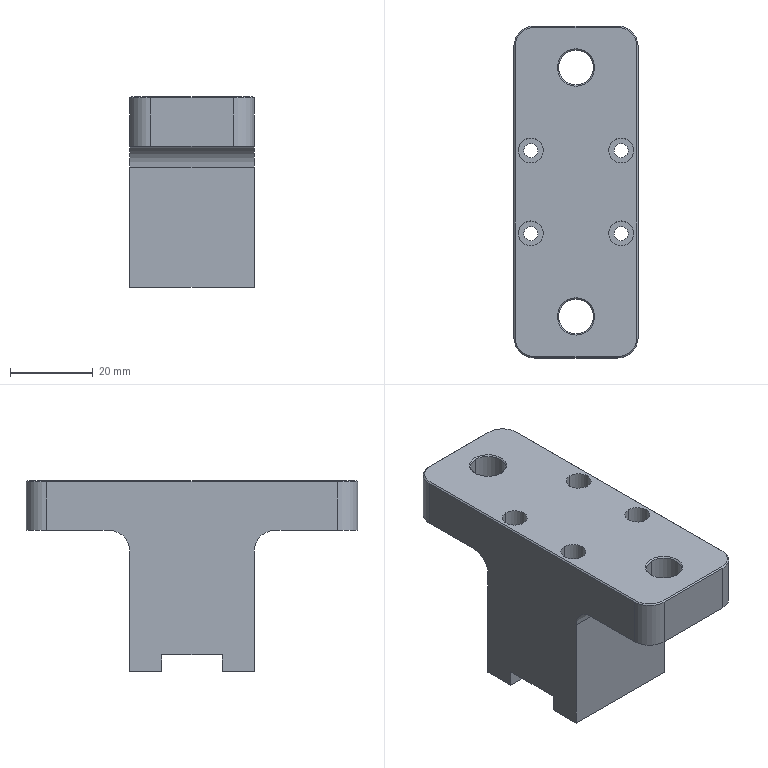NC program | NX | posted with a generic post | part box 30 x 80 x 46 mm
Lines 1 to 18 of 3641:
N10 G17 G21 G94 G90
(FLOOR_WALL_COPY , TOOL : D80)
N12 T19 M6
N14 G54
N16 G17 G0 G90 X-87. Y0. S6500 M3
N18 G43 Z30. H19
N20 Z3.
N22 G94 G1 Z0. F1500.
N24 X-82.
N26 X82.
N28 X87.
N30 Z3.
N32 G0 Z30.
N34 M5